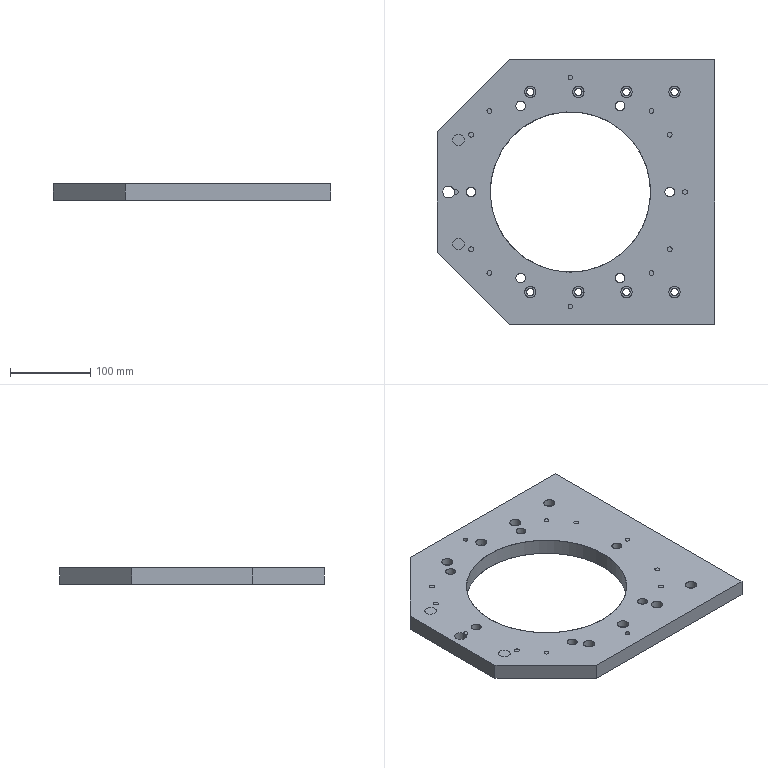NC program | NX | posted with a generic post | part box 346 x 330 x 20 mm
Lines 97 to 1013 of 28317:
(HOLE_MILLING , TOOL : D10)
N168 T10 M6
N170 G54
N172 G17 G0 G90 X-125. Y123. S3200 M3
N174 G43 Z70. H10
N176 Z0.5
N178 G94 G3 X-124. Y124. R1. F2200.
N180 X-125. Y125. R1.
N182 X-125. Y125. Z0.28 I0. J-2.
N184 X-125. Y125. Z0.06 I0. J-2.
N186 X-125. Y125. Z-0.16 I0. J-2.
N188 X-125. Y125. Z-0.38 I0. J-2.
N190 X-125. Y125. Z-0.6 I0. J-2.
N192 X-125. Y125. Z-0.82 I0. J-2.
N194 X-125. Y125. Z-1.04 I0. J-2.
N196 X-125. Y125. Z-1.26 I0. J-2.
N198 X-125. Y125. Z-1.48 I0. J-2.
N200 X-125. Y125. Z-1.7 I0. J-2.
N202 X-125. Y125. Z-1.92 I0. J-2.
N204 X-125. Y125. Z-2.14 I0. J-2.
N206 X-125. Y125. Z-2.36 I0. J-2.
N208 X-125. Y125. Z-2.58 I0. J-2.
N210 X-125. Y125. Z-2.8 I0. J-2.
N212 X-125. Y125. Z-3.02 I0. J-2.
N214 X-125. Y125. Z-3.24 I0. J-2.
N216 X-125. Y125. Z-3.46 I0. J-2.
N218 X-125. Y125. Z-3.68 I0. J-2.
N220 X-125. Y125. Z-3.9 I0. J-2.
N222 X-125. Y125. Z-4.12 I0. J-2.
N224 X-125. Y125. Z-4.34 I0. J-2.
N226 X-125. Y125. Z-4.56 I0. J-2.
N228 X-125. Y125. Z-4.78 I0. J-2.
N230 X-125. Y125. Z-5. I0. J-2.
N232 X-125. Y125. Z-5.22 I0. J-2.
N234 X-125. Y125. Z-5.44 I0. J-2.
N236 X-125. Y125. Z-5.66 I0. J-2.
N238 X-125. Y125. Z-5.88 I0. J-2.
N240 X-125. Y125. Z-6.1 I0. J-2.
N242 X-125. Y125. Z-6.32 I0. J-2.
N244 X-125. Y125. Z-6.54 I0. J-2.
N246 X-125. Y125. Z-6.76 I0. J-2.
N248 X-125. Y125. Z-6.98 I0. J-2.
N250 X-125. Y125. Z-7.2 I0. J-2.
N252 X-125. Y125. Z-7.42 I0. J-2.
N254 X-125. Y125. Z-7.64 I0. J-2.
N256 X-125. Y125. Z-7.86 I0. J-2.
N258 X-125. Y125. Z-8.08 I0. J-2.
N260 X-125. Y125. Z-8.3 I0. J-2.
N262 X-125. Y125. Z-8.52 I0. J-2.
N264 X-125. Y125. Z-8.74 I0. J-2.
N266 X-125. Y125. Z-8.96 I0. J-2.
N268 X-126.819 Y123.831 Z-9. R2.
N270 X-125.831 Y121.181 R2.
N272 X-126.819 Y123.831 R-2.
N274 X-126.325 Y122.506 R1.
N276 X-125. Y123. R1.
N278 G0 Z70.
N280 Y63.
N282 Z0.5
N284 G3 X-124. Y64. R1.
N286 X-125. Y65. R1.
N288 X-125. Y65. Z0.28 I0. J-2.
N290 X-125. Y65. Z0.06 I0. J-2.
N292 X-125. Y65. Z-0.16 I0. J-2.
N294 X-125. Y65. Z-0.38 I0. J-2.
N296 X-125. Y65. Z-0.6 I0. J-2.
N298 X-125. Y65. Z-0.82 I0. J-2.
N300 X-125. Y65. Z-1.04 I0. J-2.
N302 X-125. Y65. Z-1.26 I0. J-2.
N304 X-125. Y65. Z-1.48 I0. J-2.
N306 X-125. Y65. Z-1.7 I0. J-2.
N308 X-125. Y65. Z-1.92 I0. J-2.
N310 X-125. Y65. Z-2.14 I0. J-2.
N312 X-125. Y65. Z-2.36 I0. J-2.
N314 X-125. Y65. Z-2.58 I0. J-2.
N316 X-125. Y65. Z-2.8 I0. J-2.
N318 X-125. Y65. Z-3.02 I0. J-2.
N320 X-125. Y65. Z-3.24 I0. J-2.
N322 X-125. Y65. Z-3.46 I0. J-2.
N324 X-125. Y65. Z-3.68 I0. J-2.
N326 X-125. Y65. Z-3.9 I0. J-2.
N328 X-125. Y65. Z-4.12 I0. J-2.
N330 X-125. Y65. Z-4.34 I0. J-2.
N332 X-125. Y65. Z-4.56 I0. J-2.
N334 X-125. Y65. Z-4.78 I0. J-2.
N336 X-125. Y65. Z-5. I0. J-2.
N338 X-125. Y65. Z-5.22 I0. J-2.
N340 X-125. Y65. Z-5.44 I0. J-2.
N342 X-125. Y65. Z-5.66 I0. J-2.
N344 X-125. Y65. Z-5.88 I0. J-2.
N346 X-125. Y65. Z-6.1 I0. J-2.
N348 X-125. Y65. Z-6.32 I0. J-2.
N350 X-125. Y65. Z-6.54 I0. J-2.
N352 X-125. Y65. Z-6.76 I0. J-2.
N354 X-125. Y65. Z-6.98 I0. J-2.
N356 X-125. Y65. Z-7.2 I0. J-2.
N358 X-125. Y65. Z-7.42 I0. J-2.
N360 X-125. Y65. Z-7.64 I0. J-2.
N362 X-125. Y65. Z-7.86 I0. J-2.
N364 X-125. Y65. Z-8.08 I0. J-2.
N366 X-125. Y65. Z-8.3 I0. J-2.
N368 X-125. Y65. Z-8.52 I0. J-2.
N370 X-125. Y65. Z-8.74 I0. J-2.
N372 X-125. Y65. Z-8.96 I0. J-2.
N374 X-126.819 Y63.831 Z-9. R2.
N376 X-125.831 Y61.181 R2.
N378 X-126.819 Y63.831 R-2.
N380 X-126.325 Y62.506 R1.
N382 X-125. Y63. R1.
N384 G0 Z70.
N386 Y3.
N388 Z0.5
N390 G3 X-124. Y4. R1.
N392 X-125. Y5. R1.
N394 X-125. Y5. Z0.28 I0. J-2.
N396 X-125. Y5. Z0.06 I0. J-2.
N398 X-125. Y5. Z-0.16 I0. J-2.
N400 X-125. Y5. Z-0.38 I0. J-2.
N402 X-125. Y5. Z-0.6 I0. J-2.
N404 X-125. Y5. Z-0.82 I0. J-2.
N406 X-125. Y5. Z-1.04 I0. J-2.
N408 X-125. Y5. Z-1.26 I0. J-2.
N410 X-125. Y5. Z-1.48 I0. J-2.
N412 X-125. Y5. Z-1.7 I0. J-2.
N414 X-125. Y5. Z-1.92 I0. J-2.
N416 X-125. Y5. Z-2.14 I0. J-2.
N418 X-125. Y5. Z-2.36 I0. J-2.
N420 X-125. Y5. Z-2.58 I0. J-2.
N422 X-125. Y5. Z-2.8 I0. J-2.
N424 X-125. Y5. Z-3.02 I0. J-2.
N426 X-125. Y5. Z-3.24 I0. J-2.
N428 X-125. Y5. Z-3.46 I0. J-2.
N430 X-125. Y5. Z-3.68 I0. J-2.
N432 X-125. Y5. Z-3.9 I0. J-2.
N434 X-125. Y5. Z-4.12 I0. J-2.
N436 X-125. Y5. Z-4.34 I0. J-2.
N438 X-125. Y5. Z-4.56 I0. J-2.
N440 X-125. Y5. Z-4.78 I0. J-2.
N442 X-125. Y5. Z-5. I0. J-2.
N444 X-125. Y5. Z-5.22 I0. J-2.
N446 X-125. Y5. Z-5.44 I0. J-2.
N448 X-125. Y5. Z-5.66 I0. J-2.
N450 X-125. Y5. Z-5.88 I0. J-2.
N452 X-125. Y5. Z-6.1 I0. J-2.
N454 X-125. Y5. Z-6.32 I0. J-2.
N456 X-125. Y5. Z-6.54 I0. J-2.
N458 X-125. Y5. Z-6.76 I0. J-2.
N460 X-125. Y5. Z-6.98 I0. J-2.
N462 X-125. Y5. Z-7.2 I0. J-2.
N464 X-125. Y5. Z-7.42 I0. J-2.
N466 X-125. Y5. Z-7.64 I0. J-2.
N468 X-125. Y5. Z-7.86 I0. J-2.
N470 X-125. Y5. Z-8.08 I0. J-2.
N472 X-125. Y5. Z-8.3 I0. J-2.
N474 X-125. Y5. Z-8.52 I0. J-2.
N476 X-125. Y5. Z-8.74 I0. J-2.
N478 X-125. Y5. Z-8.96 I0. J-2.
N480 X-126.819 Y3.831 Z-9. R2.
N482 X-125.831 Y1.181 R2.
N484 X-126.819 Y3.831 R-2.
N486 X-126.325 Y2.506 R1.
N488 X-125. Y3. R1.
N490 G0 Z70.
N492 Y-57.
N494 Z0.5
N496 G3 X-124. Y-56. R1.
N498 X-125. Y-55. R1.
N500 X-125. Y-55. Z0.28 I0. J-2.
N502 X-125. Y-55. Z0.06 I0. J-2.
N504 X-125. Y-55. Z-0.16 I0. J-2.
N506 X-125. Y-55. Z-0.38 I0. J-2.
N508 X-125. Y-55. Z-0.6 I0. J-2.
N510 X-125. Y-55. Z-0.82 I0. J-2.
N512 X-125. Y-55. Z-1.04 I0. J-2.
N514 X-125. Y-55. Z-1.26 I0. J-2.
N516 X-125. Y-55. Z-1.48 I0. J-2.
N518 X-125. Y-55. Z-1.7 I0. J-2.
N520 X-125. Y-55. Z-1.92 I0. J-2.
N522 X-125. Y-55. Z-2.14 I0. J-2.
N524 X-125. Y-55. Z-2.36 I0. J-2.
N526 X-125. Y-55. Z-2.58 I0. J-2.
N528 X-125. Y-55. Z-2.8 I0. J-2.
N530 X-125. Y-55. Z-3.02 I0. J-2.
N532 X-125. Y-55. Z-3.24 I0. J-2.
N534 X-125. Y-55. Z-3.46 I0. J-2.
N536 X-125. Y-55. Z-3.68 I0. J-2.
N538 X-125. Y-55. Z-3.9 I0. J-2.
N540 X-125. Y-55. Z-4.12 I0. J-2.
N542 X-125. Y-55. Z-4.34 I0. J-2.
N544 X-125. Y-55. Z-4.56 I0. J-2.
N546 X-125. Y-55. Z-4.78 I0. J-2.
N548 X-125. Y-55. Z-5. I0. J-2.
N550 X-125. Y-55. Z-5.22 I0. J-2.
N552 X-125. Y-55. Z-5.44 I0. J-2.
N554 X-125. Y-55. Z-5.66 I0. J-2.
N556 X-125. Y-55. Z-5.88 I0. J-2.
N558 X-125. Y-55. Z-6.1 I0. J-2.
N560 X-125. Y-55. Z-6.32 I0. J-2.
N562 X-125. Y-55. Z-6.54 I0. J-2.
N564 X-125. Y-55. Z-6.76 I0. J-2.
N566 X-125. Y-55. Z-6.98 I0. J-2.
N568 X-125. Y-55. Z-7.2 I0. J-2.
N570 X-125. Y-55. Z-7.42 I0. J-2.
N572 X-125. Y-55. Z-7.64 I0. J-2.
N574 X-125. Y-55. Z-7.86 I0. J-2.
N576 X-125. Y-55. Z-8.08 I0. J-2.
N578 X-125. Y-55. Z-8.3 I0. J-2.
N580 X-125. Y-55. Z-8.52 I0. J-2.
N582 X-125. Y-55. Z-8.74 I0. J-2.
N584 X-125. Y-55. Z-8.96 I0. J-2.
N586 X-126.819 Y-56.169 Z-9. R2.
N588 X-125.831 Y-58.819 R2.
N590 X-126.819 Y-56.169 R-2.
N592 X-126.325 Y-57.494 R1.
N594 X-125. Y-57. R1.
N596 G0 Z70.
N598 X125.
N600 Z0.5
N602 G3 X126. Y-56. R1.
N604 X125. Y-55. R1.
N606 X125. Y-55. Z0.28 I0. J-2.
N608 X125. Y-55. Z0.06 I0. J-2.
N610 X125. Y-55. Z-0.16 I0. J-2.
N612 X125. Y-55. Z-0.38 I0. J-2.
N614 X125. Y-55. Z-0.6 I0. J-2.
N616 X125. Y-55. Z-0.82 I0. J-2.
N618 X125. Y-55. Z-1.04 I0. J-2.
N620 X125. Y-55. Z-1.26 I0. J-2.
N622 X125. Y-55. Z-1.48 I0. J-2.
N624 X125. Y-55. Z-1.7 I0. J-2.
N626 X125. Y-55. Z-1.92 I0. J-2.
N628 X125. Y-55. Z-2.14 I0. J-2.
N630 X125. Y-55. Z-2.36 I0. J-2.
N632 X125. Y-55. Z-2.58 I0. J-2.
N634 X125. Y-55. Z-2.8 I0. J-2.
N636 X125. Y-55. Z-3.02 I0. J-2.
N638 X125. Y-55. Z-3.24 I0. J-2.
N640 X125. Y-55. Z-3.46 I0. J-2.
N642 X125. Y-55. Z-3.68 I0. J-2.
N644 X125. Y-55. Z-3.9 I0. J-2.
N646 X125. Y-55. Z-4.12 I0. J-2.
N648 X125. Y-55. Z-4.34 I0. J-2.
N650 X125. Y-55. Z-4.56 I0. J-2.
N652 X125. Y-55. Z-4.78 I0. J-2.
N654 X125. Y-55. Z-5. I0. J-2.
N656 X125. Y-55. Z-5.22 I0. J-2.
N658 X125. Y-55. Z-5.44 I0. J-2.
N660 X125. Y-55. Z-5.66 I0. J-2.
N662 X125. Y-55. Z-5.88 I0. J-2.
N664 X125. Y-55. Z-6.1 I0. J-2.
N666 X125. Y-55. Z-6.32 I0. J-2.
N668 X125. Y-55. Z-6.54 I0. J-2.
N670 X125. Y-55. Z-6.76 I0. J-2.
N672 X125. Y-55. Z-6.98 I0. J-2.
N674 X125. Y-55. Z-7.2 I0. J-2.
N676 X125. Y-55. Z-7.42 I0. J-2.
N678 X125. Y-55. Z-7.64 I0. J-2.
N680 X125. Y-55. Z-7.86 I0. J-2.
N682 X125. Y-55. Z-8.08 I0. J-2.
N684 X125. Y-55. Z-8.3 I0. J-2.
N686 X125. Y-55. Z-8.52 I0. J-2.
N688 X125. Y-55. Z-8.74 I0. J-2.
N690 X125. Y-55. Z-8.96 I0. J-2.
N692 X123.181 Y-56.169 Z-9. R2.
N694 X124.169 Y-58.819 R2.
N696 X123.181 Y-56.169 R-2.
N698 X123.675 Y-57.494 R1.
N700 X125. Y-57. R1.
N702 G0 Z70.
N704 Y3.
N706 Z0.5
N708 G3 X126. Y4. R1.
N710 X125. Y5. R1.
N712 X125. Y5. Z0.28 I0. J-2.
N714 X125. Y5. Z0.06 I0. J-2.
N716 X125. Y5. Z-0.16 I0. J-2.
N718 X125. Y5. Z-0.38 I0. J-2.
N720 X125. Y5. Z-0.6 I0. J-2.
N722 X125. Y5. Z-0.82 I0. J-2.
N724 X125. Y5. Z-1.04 I0. J-2.
N726 X125. Y5. Z-1.26 I0. J-2.
N728 X125. Y5. Z-1.48 I0. J-2.
N730 X125. Y5. Z-1.7 I0. J-2.
N732 X125. Y5. Z-1.92 I0. J-2.
N734 X125. Y5. Z-2.14 I0. J-2.
N736 X125. Y5. Z-2.36 I0. J-2.
N738 X125. Y5. Z-2.58 I0. J-2.
N740 X125. Y5. Z-2.8 I0. J-2.
N742 X125. Y5. Z-3.02 I0. J-2.
N744 X125. Y5. Z-3.24 I0. J-2.
N746 X125. Y5. Z-3.46 I0. J-2.
N748 X125. Y5. Z-3.68 I0. J-2.
N750 X125. Y5. Z-3.9 I0. J-2.
N752 X125. Y5. Z-4.12 I0. J-2.
N754 X125. Y5. Z-4.34 I0. J-2.
N756 X125. Y5. Z-4.56 I0. J-2.
N758 X125. Y5. Z-4.78 I0. J-2.
N760 X125. Y5. Z-5. I0. J-2.
N762 X125. Y5. Z-5.22 I0. J-2.
N764 X125. Y5. Z-5.44 I0. J-2.
N766 X125. Y5. Z-5.66 I0. J-2.
N768 X125. Y5. Z-5.88 I0. J-2.
N770 X125. Y5. Z-6.1 I0. J-2.
N772 X125. Y5. Z-6.32 I0. J-2.
N774 X125. Y5. Z-6.54 I0. J-2.
N776 X125. Y5. Z-6.76 I0. J-2.
N778 X125. Y5. Z-6.98 I0. J-2.
N780 X125. Y5. Z-7.2 I0. J-2.
N782 X125. Y5. Z-7.42 I0. J-2.
N784 X125. Y5. Z-7.64 I0. J-2.
N786 X125. Y5. Z-7.86 I0. J-2.
N788 X125. Y5. Z-8.08 I0. J-2.
N790 X125. Y5. Z-8.3 I0. J-2.
N792 X125. Y5. Z-8.52 I0. J-2.
N794 X125. Y5. Z-8.74 I0. J-2.
N796 X125. Y5. Z-8.96 I0. J-2.
N798 X123.181 Y3.831 Z-9. R2.
N800 X124.169 Y1.181 R2.
N802 X123.181 Y3.831 R-2.
N804 X123.675 Y2.506 R1.
N806 X125. Y3. R1.
N808 G0 Z70.
N810 Y63.
N812 Z0.5
N814 G3 X126. Y64. R1.
N816 X125. Y65. R1.
N818 X125. Y65. Z0.28 I0. J-2.
N820 X125. Y65. Z0.06 I0. J-2.
N822 X125. Y65. Z-0.16 I0. J-2.
N824 X125. Y65. Z-0.38 I0. J-2.
N826 X125. Y65. Z-0.6 I0. J-2.
N828 X125. Y65. Z-0.82 I0. J-2.
N830 X125. Y65. Z-1.04 I0. J-2.
N832 X125. Y65. Z-1.26 I0. J-2.
N834 X125. Y65. Z-1.48 I0. J-2.
N836 X125. Y65. Z-1.7 I0. J-2.
N838 X125. Y65. Z-1.92 I0. J-2.
N840 X125. Y65. Z-2.14 I0. J-2.
N842 X125. Y65. Z-2.36 I0. J-2.
N844 X125. Y65. Z-2.58 I0. J-2.
N846 X125. Y65. Z-2.8 I0. J-2.
N848 X125. Y65. Z-3.02 I0. J-2.
N850 X125. Y65. Z-3.24 I0. J-2.
N852 X125. Y65. Z-3.46 I0. J-2.
N854 X125. Y65. Z-3.68 I0. J-2.
N856 X125. Y65. Z-3.9 I0. J-2.
N858 X125. Y65. Z-4.12 I0. J-2.
N860 X125. Y65. Z-4.34 I0. J-2.
N862 X125. Y65. Z-4.56 I0. J-2.
N864 X125. Y65. Z-4.78 I0. J-2.
N866 X125. Y65. Z-5. I0. J-2.
N868 X125. Y65. Z-5.22 I0. J-2.
N870 X125. Y65. Z-5.44 I0. J-2.
N872 X125. Y65. Z-5.66 I0. J-2.
N874 X125. Y65. Z-5.88 I0. J-2.
N876 X125. Y65. Z-6.1 I0. J-2.
N878 X125. Y65. Z-6.32 I0. J-2.
N880 X125. Y65. Z-6.54 I0. J-2.
N882 X125. Y65. Z-6.76 I0. J-2.
N884 X125. Y65. Z-6.98 I0. J-2.
N886 X125. Y65. Z-7.2 I0. J-2.
N888 X125. Y65. Z-7.42 I0. J-2.
N890 X125. Y65. Z-7.64 I0. J-2.
N892 X125. Y65. Z-7.86 I0. J-2.
N894 X125. Y65. Z-8.08 I0. J-2.
N896 X125. Y65. Z-8.3 I0. J-2.
N898 X125. Y65. Z-8.52 I0. J-2.
N900 X125. Y65. Z-8.74 I0. J-2.
N902 X125. Y65. Z-8.96 I0. J-2.
N904 X123.181 Y63.831 Z-9. R2.
N906 X124.169 Y61.181 R2.
N908 X123.181 Y63.831 R-2.
N910 X123.675 Y62.506 R1.
N912 X125. Y63. R1.
N914 G0 Z70.
N916 Y123.
N918 Z0.5
N920 G3 X126. Y124. R1.
N922 X125. Y125. R1.
N924 X125. Y125. Z0.28 I0. J-2.
N926 X125. Y125. Z0.06 I0. J-2.
N928 X125. Y125. Z-0.16 I0. J-2.
N930 X125. Y125. Z-0.38 I0. J-2.
N932 X125. Y125. Z-0.6 I0. J-2.
N934 X125. Y125. Z-0.82 I0. J-2.
N936 X125. Y125. Z-1.04 I0. J-2.
N938 X125. Y125. Z-1.26 I0. J-2.
N940 X125. Y125. Z-1.48 I0. J-2.
N942 X125. Y125. Z-1.7 I0. J-2.
N944 X125. Y125. Z-1.92 I0. J-2.
N946 X125. Y125. Z-2.14 I0. J-2.
N948 X125. Y125. Z-2.36 I0. J-2.
N950 X125. Y125. Z-2.58 I0. J-2.
N952 X125. Y125. Z-2.8 I0. J-2.
N954 X125. Y125. Z-3.02 I0. J-2.
N956 X125. Y125. Z-3.24 I0. J-2.
N958 X125. Y125. Z-3.46 I0. J-2.
N960 X125. Y125. Z-3.68 I0. J-2.
N962 X125. Y125. Z-3.9 I0. J-2.
N964 X125. Y125. Z-4.12 I0. J-2.
N966 X125. Y125. Z-4.34 I0. J-2.
N968 X125. Y125. Z-4.56 I0. J-2.
N970 X125. Y125. Z-4.78 I0. J-2.
N972 X125. Y125. Z-5. I0. J-2.
N974 X125. Y125. Z-5.22 I0. J-2.
N976 X125. Y125. Z-5.44 I0. J-2.
N978 X125. Y125. Z-5.66 I0. J-2.
N980 X125. Y125. Z-5.88 I0. J-2.
N982 X125. Y125. Z-6.1 I0. J-2.
N984 X125. Y125. Z-6.32 I0. J-2.
N986 X125. Y125. Z-6.54 I0. J-2.
N988 X125. Y125. Z-6.76 I0. J-2.
N990 X125. Y125. Z-6.98 I0. J-2.
N992 X125. Y125. Z-7.2 I0. J-2.
N994 X125. Y125. Z-7.42 I0. J-2.
N996 X125. Y125. Z-7.64 I0. J-2.
N998 X125. Y125. Z-7.86 I0. J-2.
N1000 X125. Y125. Z-8.08 I0. J-2.
N1002 X125. Y125. Z-8.3 I0. J-2.
N1004 X125. Y125. Z-8.52 I0. J-2.
N1006 X125. Y125. Z-8.74 I0. J-2.
N1008 X125. Y125. Z-8.96 I0. J-2.
N1010 X123.181 Y123.831 Z-9. R2.
N1012 X124.169 Y121.181 R2.
N1014 X123.181 Y123.831 R-2.
N1016 X123.675 Y122.506 R1.
N1018 X125. Y123. R1.
N1020 G0 Z70.
(ZLEVEL_PROFILE , TOOL : D10)
N1022 X-173.211 Y182.777 S2200
N1024 Z2.78
N1026 G1 Z-0.22
N1028 X-170.826 Y178.649
N1030 G3 X-169.96 Y178.149 R1.
N1032 G1 X-165.039 Y178.15
N1034 X160.475
N1036 X169.96 Y178.149
N1038 G3 X170.826 Y178.649 R1.
N1040 G1 X173.212 Y182.781
N1042 Z2.78
N1044 G0 Z2.56
N1046 G1 Z-0.44
N1048 X170.826 Y178.649
N1050 G2 X169.96 Y178.149 R1.
N1052 G1 X160.475 Y178.15
N1054 X-165.039
N1056 X-169.96 Y178.149
N1058 G2 X-170.826 Y178.649 R1.
N1060 G1 X-173.211 Y182.777
N1062 Z2.56
N1064 G0 Z2.341
N1066 G1 Z-0.659
N1068 X-170.826 Y178.649
N1070 G3 X-169.96 Y178.149 R1.
N1072 G1 X-165.039 Y178.15
N1074 X160.475
N1076 X169.96 Y178.149
N1078 G3 X170.826 Y178.649 R1.
N1080 G1 X173.212 Y182.781
N1082 Z2.341
N1084 G0 Z2.121
N1086 G1 Z-0.879
N1088 X170.826 Y178.649
N1090 G2 X169.96 Y178.149 R1.
N1092 G1 X160.475 Y178.15
N1094 X-165.039
N1096 X-169.96 Y178.149
N1098 G2 X-170.826 Y178.649 R1.
N1100 G1 X-173.211 Y182.777
N1102 Z2.121
N1104 G0 Z1.901
N1106 G1 Z-1.099
N1108 X-170.826 Y178.649
N1110 G3 X-169.96 Y178.149 R1.
N1112 G1 X-165.039 Y178.15
N1114 X160.475
N1116 X169.96 Y178.149
N1118 G3 X170.826 Y178.649 R1.
N1120 G1 X173.212 Y182.781
N1122 Z1.901
N1124 G0 Z1.681
N1126 G1 Z-1.319
N1128 X170.826 Y178.649
N1130 G2 X169.96 Y178.149 R1.
N1132 G1 X160.475 Y178.15
N1134 X-165.039
N1136 X-169.96 Y178.149
N1138 G2 X-170.826 Y178.649 R1.
N1140 G1 X-173.211 Y182.777
N1142 Z1.681
N1144 G0 Z1.462
N1146 G1 Z-1.538
N1148 X-170.826 Y178.649
N1150 G3 X-169.96 Y178.149 R1.
N1152 G1 X-165.039 Y178.15
N1154 X160.475
N1156 X169.96 Y178.149
N1158 G3 X170.826 Y178.649 R1.
N1160 G1 X173.212 Y182.781
N1162 Z1.462
N1164 G0 Z1.242
N1166 G1 Z-1.758
N1168 X170.826 Y178.649
N1170 G2 X169.96 Y178.149 R1.
N1172 G1 X160.475 Y178.15
N1174 X-165.039
N1176 X-169.96 Y178.149
N1178 G2 X-170.826 Y178.649 R1.
N1180 G1 X-173.211 Y182.777
N1182 Z1.242
N1184 G0 Z1.022
N1186 G1 Z-1.978
N1188 X-170.826 Y178.649
N1190 G3 X-169.96 Y178.149 R1.
N1192 G1 X-165.039 Y178.15
N1194 X160.475
N1196 X169.96 Y178.149
N1198 G3 X170.826 Y178.649 R1.
N1200 G1 X173.212 Y182.781
N1202 Z1.022
N1204 G0 Z0.802
N1206 G1 Z-2.198
N1208 X170.826 Y178.649
N1210 G2 X169.96 Y178.149 R1.
N1212 G1 X160.475 Y178.15
N1214 X-165.039
N1216 X-169.96 Y178.149
N1218 G2 X-170.826 Y178.649 R1.
N1220 G1 X-173.211 Y182.777
N1222 Z0.802
N1224 G0 Z0.582
N1226 G1 Z-2.418
N1228 X-170.826 Y178.649
N1230 G3 X-169.96 Y178.149 R1.
N1232 G1 X-165.039 Y178.15
N1234 X160.475
N1236 X169.96 Y178.149
N1238 G3 X170.826 Y178.649 R1.
N1240 G1 X173.212 Y182.781
N1242 Z0.582
N1244 G0 Z0.363
N1246 G1 Z-2.637
N1248 X170.826 Y178.649
N1250 G2 X169.96 Y178.149 R1.
N1252 G1 X160.475 Y178.15
N1254 X-165.039
N1256 X-169.96 Y178.149
N1258 G2 X-170.826 Y178.649 R1.
N1260 G1 X-173.211 Y182.777
N1262 Z0.363
N1264 G0 Z0.143
N1266 G1 Z-2.857
N1268 X-170.826 Y178.649
N1270 G3 X-169.96 Y178.149 R1.
N1272 G1 X-165.039 Y178.15
N1274 X160.475
N1276 X169.96 Y178.149
N1278 G3 X170.826 Y178.649 R1.
N1280 G1 X173.212 Y182.781
N1282 Z0.143
N1284 G0 Z-0.077
N1286 G1 Z-3.077
N1288 X170.826 Y178.649
N1290 G2 X169.96 Y178.149 R1.
N1292 G1 X160.475 Y178.15
N1294 X-165.039
N1296 X-169.96 Y178.149
N1298 G2 X-170.826 Y178.649 R1.
N1300 G1 X-173.211 Y182.777
N1302 Z-0.077
N1304 G0 Z-0.297
N1306 G1 Z-3.297
N1308 X-170.826 Y178.649
N1310 G3 X-169.96 Y178.149 R1.
N1312 G1 X-165.039 Y178.15
N1314 X160.475
N1316 X169.96 Y178.149
N1318 G3 X170.826 Y178.649 R1.
N1320 G1 X173.212 Y182.781
N1322 Z-0.297
N1324 G0 Z-0.516
N1326 G1 Z-3.516
N1328 X170.826 Y178.649
N1330 G2 X169.96 Y178.149 R1.
N1332 G1 X160.475 Y178.15
N1334 X-165.039
N1336 X-169.96 Y178.149
N1338 G2 X-170.826 Y178.649 R1.
N1340 G1 X-173.211 Y182.777
N1342 Z-0.516
N1344 G0 X-173.21 Z-0.736
N1346 G1 Z-3.736
N1348 X-170.826 Y178.649
N1350 G3 X-169.96 Y178.149 R1.
N1352 G1 X-165.039 Y178.15
N1354 X160.475
N1356 X169.96 Y178.149
N1358 G3 X170.826 Y178.649 R1.
N1360 G1 X173.212 Y182.781
N1362 Z-0.736
N1364 G0 Z-0.956
N1366 G1 Z-3.956
N1368 X170.826 Y178.649
N1370 G2 X169.96 Y178.149 R1.
N1372 G1 X160.475 Y178.15
N1374 X-165.039
N1376 X-169.96 Y178.149
N1378 G2 X-170.826 Y178.649 R1.
N1380 G1 X-173.21 Y182.777
N1382 Z-0.956
N1384 G0 Z-1.176
N1386 G1 Z-4.176
N1388 X-170.826 Y178.649
N1390 G3 X-169.96 Y178.149 R1.
N1392 G1 X-165.039 Y178.15
N1394 X160.475
N1396 X169.96 Y178.149
N1398 G3 X170.826 Y178.649 R1.
N1400 G1 X173.212 Y182.781
N1402 Z-1.176
N1404 G0 Z-1.396
N1406 G1 Z-4.396
N1408 X170.826 Y178.649
N1410 G2 X169.96 Y178.149 R1.
N1412 G1 X160.475 Y178.15
N1414 X-165.039
N1416 X-169.96 Y178.149
N1418 G2 X-170.826 Y178.649 R1.
N1420 G1 X-173.21 Y182.777
N1422 Z-1.396
N1424 G0 Z-1.615
N1426 G1 Z-4.615
N1428 X-170.826 Y178.649
N1430 G3 X-169.96 Y178.149 R1.
N1432 G1 X-165.039 Y178.15
N1434 X160.475
N1436 X169.96 Y178.149
N1438 G3 X170.826 Y178.649 R1.
N1440 G1 X173.212 Y182.781
N1442 Z-1.615
N1444 G0 Z-1.835
N1446 G1 Z-4.835
N1448 X170.826 Y178.649
N1450 G2 X169.96 Y178.149 R1.
N1452 G1 X160.475 Y178.15
N1454 X-165.039
N1456 X-169.96 Y178.149
N1458 G2 X-170.826 Y178.649 R1.
N1460 G1 X-173.21 Y182.777
N1462 Z-1.835
N1464 G0 Z-2.055
N1466 G1 Z-5.055
N1468 X-170.826 Y178.649
N1470 G3 X-169.96 Y178.149 R1.
N1472 G1 X-165.039 Y178.15
N1474 X160.475
N1476 X169.96 Y178.149
N1478 G3 X170.826 Y178.649 R1.
N1480 G1 X173.212 Y182.781
N1482 Z-2.055
N1484 G0 Z-2.275
N1486 G1 Z-5.275
N1488 X170.826 Y178.649
N1490 G2 X169.96 Y178.149 R1.
N1492 G1 X160.475 Y178.15
N1494 X-165.039
N1496 X-169.96 Y178.149
N1498 G2 X-170.826 Y178.649 R1.
N1500 G1 X-173.21 Y182.777
N1502 Z-2.275
N1504 G0 Z-2.495
N1506 G1 Z-5.495
N1508 X-170.826 Y178.649
N1510 G3 X-169.96 Y178.149 R1.
N1512 G1 X-165.039 Y178.15
N1514 X160.475
N1516 X169.96 Y178.149
N1518 G3 X170.826 Y178.649 R1.
N1520 G1 X173.212 Y182.781
N1522 Z-2.495
N1524 G0 Z-2.714
N1526 G1 Z-5.714
N1528 X170.826 Y178.649
N1530 G2 X169.96 Y178.149 R1.
N1532 G1 X160.475 Y178.15
N1534 X-165.039
N1536 X-169.96 Y178.149
N1538 G2 X-170.826 Y178.649 R1.
N1540 G1 X-173.21 Y182.777
N1542 Z-2.714
N1544 G0 Z-2.934
N1546 G1 Z-5.934
N1548 X-170.826 Y178.649
N1550 G3 X-169.96 Y178.149 R1.
N1552 G1 X-165.039 Y178.15
N1554 X160.475
N1556 X169.96 Y178.149
N1558 G3 X170.826 Y178.649 R1.
N1560 G1 X173.212 Y182.781
N1562 Z-2.934
N1564 G0 Z-3.154
N1566 G1 Z-6.154
N1568 X170.826 Y178.649
N1570 G2 X169.96 Y178.149 R1.
N1572 G1 X160.475 Y178.15
N1574 X-165.039
N1576 X-169.96 Y178.149
N1578 G2 X-170.826 Y178.649 R1.
N1580 G1 X-173.21 Y182.777
N1582 Z-3.154
N1584 G0 Z-3.374
N1586 G1 Z-6.374
N1588 X-170.826 Y178.649
N1590 G3 X-169.96 Y178.149 R1.
N1592 G1 X-165.039 Y178.15
N1594 X160.475
N1596 X169.96 Y178.149
N1598 G3 X170.826 Y178.649 R1.
N1600 G1 X173.212 Y182.781
N1602 Z-3.374
N1604 G0 Z-3.593
N1606 G1 Z-6.593
N1608 X170.826 Y178.649
N1610 G2 X169.96 Y178.149 R1.
N1612 G1 X160.475 Y178.15
N1614 X-165.039
N1616 X-169.96 Y178.149
N1618 G2 X-170.826 Y178.649 R1.
N1620 G1 X-173.21 Y182.777
N1622 Z-3.593
N1624 G0 Z-3.813
N1626 G1 Z-6.813
N1628 X-170.826 Y178.649
N1630 G3 X-169.96 Y178.149 R1.
N1632 G1 X-165.039 Y178.15
N1634 X160.475
N1636 X169.96 Y178.149
N1638 G3 X170.826 Y178.649 R1.
N1640 G1 X173.212 Y182.781
N1642 Z-3.813
N1644 G0 Z-4.033
N1646 G1 Z-7.033
N1648 X170.826 Y178.649
N1650 G2 X169.96 Y178.149 R1.
N1652 G1 X160.475 Y178.15
N1654 X-165.039
N1656 X-169.96 Y178.149
N1658 G2 X-170.826 Y178.649 R1.
N1660 G1 X-173.21 Y182.777
N1662 Z-4.033
N1664 G0 Z-4.253
N1666 G1 Z-7.253
N1668 X-170.826 Y178.649
N1670 G3 X-169.96 Y178.149 R1.
N1672 G1 X-165.039 Y178.15
N1674 X160.475
N1676 X169.96 Y178.149
N1678 G3 X170.826 Y178.649 R1.
N1680 G1 X173.212 Y182.781
N1682 Z-4.253
N1684 G0 Z-4.473
N1686 G1 Z-7.473
N1688 X170.826 Y178.649
N1690 G2 X169.96 Y178.149 R1.
N1692 G1 X160.475 Y178.15
N1694 X-165.039
N1696 X-169.96 Y178.149
N1698 G2 X-170.826 Y178.649 R1.
N1700 G1 X-173.21 Y182.777
N1702 Z-4.473
N1704 G0 Z-4.692
N1706 G1 Z-7.692
N1708 X-170.826 Y178.649
N1710 G3 X-169.96 Y178.149 R1.
N1712 G1 X-165.039 Y178.15
N1714 X160.475
N1716 X169.96 Y178.149
N1718 G3 X170.826 Y178.649 R1.
N1720 G1 X173.212 Y182.781
N1722 Z-4.692
N1724 G0 Y182.782 Z-4.912
N1726 G1 Z-7.912
N1728 X170.826 Y178.649
N1730 G2 X169.96 Y178.149 R1.
N1732 G1 X160.475 Y178.15
N1734 X-165.039
N1736 X-169.96 Y178.149
N1738 G2 X-170.826 Y178.649 R1.
N1740 G1 X-173.21 Y182.777
N1742 Z-4.912
N1744 G0 Z-5.132
N1746 G1 Z-8.132
N1748 X-170.826 Y178.649
N1750 G3 X-169.96 Y178.149 R1.
N1752 G1 X-165.039 Y178.15
N1754 X160.475
N1756 X169.96 Y178.149
N1758 G3 X170.826 Y178.649 R1.
N1760 G1 X173.212 Y182.782
N1762 Z-5.132
N1764 G0 Z-5.352
N1766 G1 Z-8.352
N1768 X170.826 Y178.649
N1770 G2 X169.96 Y178.149 R1.
N1772 G1 X160.475 Y178.15
N1774 X-165.039
N1776 X-169.96 Y178.149
N1778 G2 X-170.826 Y178.649 R1.
N1780 G1 X-173.21 Y182.777
N1782 Z-5.352
N1784 G0 Z-5.571
N1786 G1 Z-8.571
N1788 X-170.826 Y178.649
N1790 G3 X-169.96 Y178.149 R1.
N1792 G1 X-165.039 Y178.15
N1794 X160.475
N1796 X169.96 Y178.149
N1798 G3 X170.826 Y178.649 R1.
N1800 G1 X173.212 Y182.782
N1802 Z-5.571
N1804 G0 Z-5.791
N1806 G1 Z-8.791
N1808 X170.826 Y178.649
N1810 G2 X169.96 Y178.149 R1.
N1812 G1 X160.475 Y178.15
N1814 X-165.039
N1816 X-169.96 Y178.149
N1818 G2 X-170.826 Y178.649 R1.
N1820 G1 X-173.21 Y182.777
N1822 Z-5.791
N1824 G0 Z-6.011
N1826 G1 Z-9.011
N1828 X-170.826 Y178.649
N1830 G3 X-169.96 Y178.149 R1.
N1832 G1 X-165.039 Y178.15
N1834 X160.475
N1836 X169.96 Y178.149
N1838 G3 X170.826 Y178.649 R1.
N1840 G1 X173.212 Y182.782
N1842 Z-6.011
N1844 G0 Z-6.231
N1846 G1 Z-9.231
N1848 X170.826 Y178.649
N1850 G2 X169.96 Y178.149 R1.
N1852 G1 X160.475 Y178.15
N1854 X-165.039
N1856 X-169.96 Y178.149
N1858 G2 X-170.826 Y178.649 R1.
N1860 G1 X-173.21 Y182.777
N1862 Z-6.231
N1864 G0 Z-6.451
N1866 G1 Z-9.451
N1868 X-170.826 Y178.649
N1870 G3 X-169.96 Y178.149 R1.
N1872 G1 X-165.039 Y178.15
N1874 X160.475
N1876 X169.96 Y178.149
N1878 G3 X170.826 Y178.649 R1.
N1880 G1 X173.212 Y182.782
N1882 Z-6.451
N1884 G0 Z-6.67
N1886 G1 Z-9.67
N1888 X170.826 Y178.649
N1890 G2 X169.96 Y178.149 R1.
N1892 G1 X160.475 Y178.15
N1894 X-165.039
N1896 X-169.96 Y178.149
N1898 G2 X-170.826 Y178.649 R1.
N1900 G1 X-173.21 Y182.777
N1902 Z-6.67
N1904 G0 Z-6.89
N1906 G1 Z-9.89
N1908 X-170.826 Y178.649
N1910 G3 X-169.96 Y178.149 R1.
N1912 G1 X-165.039 Y178.15
N1914 X160.475
N1916 X169.96 Y178.149
N1918 G3 X170.826 Y178.649 R1.
N1920 G1 X173.212 Y182.782
N1922 Z-6.89
N1924 G0 Z-7.11
N1926 G1 Z-10.11
N1928 X170.826 Y178.649
N1930 G2 X169.96 Y178.149 R1.
N1932 G1 X160.475 Y178.15
N1934 X-165.039
N1936 X-169.96 Y178.149
N1938 G2 X-170.826 Y178.649 R1.
N1940 G1 X-173.21 Y182.777
N1942 Z-7.11
N1944 G0 Z-7.33
N1946 G1 Z-10.33
N1948 X-170.826 Y178.649
N1950 G3 X-169.96 Y178.149 R1.
N1952 G1 X-165.039 Y178.15
N1954 X160.475
N1956 X169.96 Y178.149
N1958 G3 X170.826 Y178.649 R1.
N1960 G1 X173.212 Y182.782
N1962 Z-7.33
N1964 G0 Z-7.549
N1966 G1 Z-10.549
N1968 X170.826 Y178.649
N1970 G2 X169.96 Y178.149 R1.
N1972 G1 X160.475 Y178.15
N1974 X-165.039
N1976 X-169.96 Y178.149
N1978 G2 X-170.826 Y178.649 R1.
N1980 G1 X-173.21 Y182.777
N1982 Z-7.549
N1984 G0 Z-7.769
N1986 G1 Z-10.769
N1988 X-170.826 Y178.649